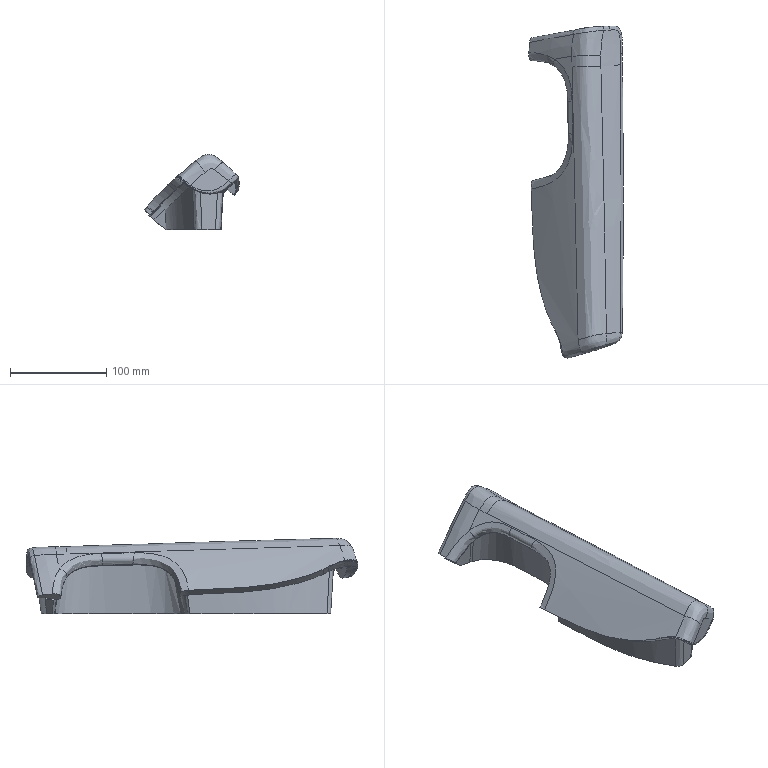Part | STEP file | 4-20.sldasm-Part-375 | 1 solid | 155 faces | box 98.33 x 345.843 x 78.457 mm | volume 972518 mm3 | spline 138 | plane 13 | cylinder 4 | commonest cylinder face diameters 6 x4